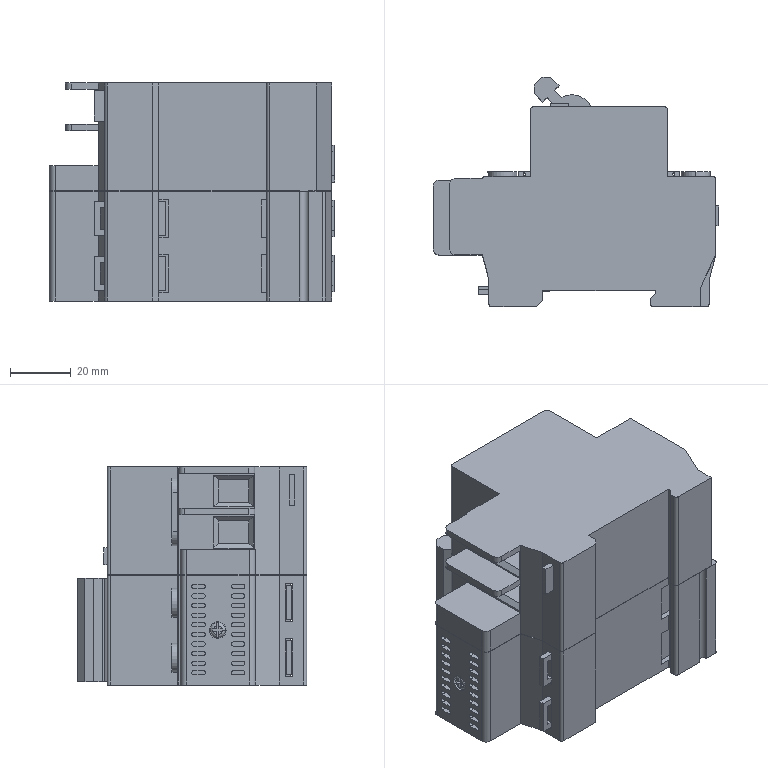Part | STEP file | NXBLE-32 2P C20 30MA 6KA | 5 solids | 648 faces | box 93.6 x 75.273 x 71.5 mm | volume 301001 mm3 | plane 477 | cylinder 168 | torus 3 | commonest cylinder face diameters 1.4 x60 5.6 x16 6.5 x12 7 x12 2 x11 3 x10